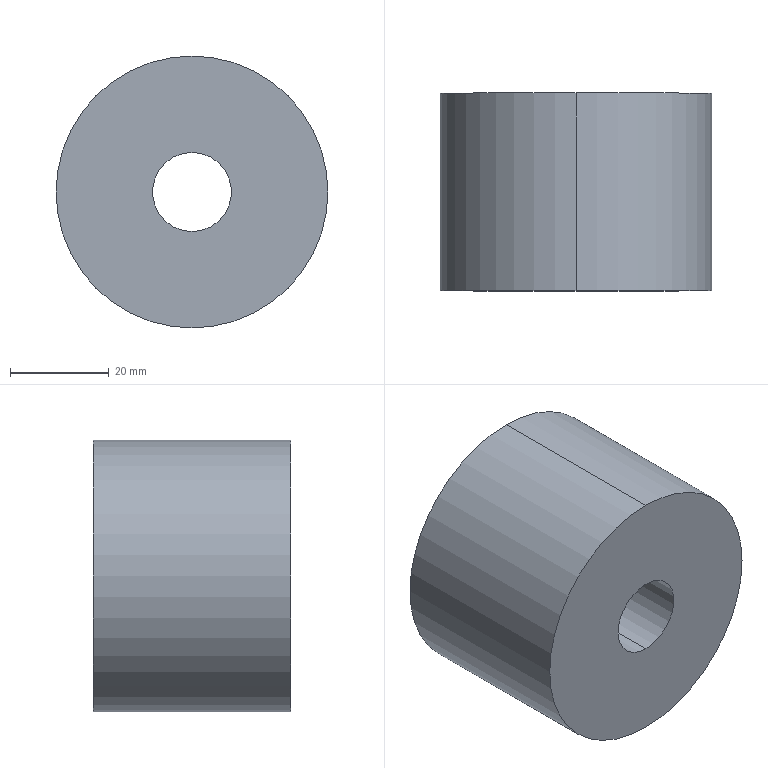Part | STEP file | 19-Limit post | 1 solid | 6 faces | box 55 x 40 x 55 mm | volume 86991 mm3 | cylinder 4 | plane 2 | commonest cylinder face diameters 16 x2 55 x2
STEP:
#1=CARTESIAN_POINT('',(0.,0.,0.));
#2=DIRECTION('',(0.,0.,1.));
#3=DIRECTION('',(1.,0.,0.));
#4=AXIS2_PLACEMENT_3D('',#1,#2,#3);
#5=CARTESIAN_POINT('',(0.,40.,-8.));
#6=VERTEX_POINT('',#5);
#7=CARTESIAN_POINT('',(0.,0.,-8.));
#8=VERTEX_POINT('',#7);
#9=CARTESIAN_POINT('',(0.,40.,-8.));
#10=DIRECTION('',(0.,-1.,0.));
#11=VECTOR('',#10,1.);
#12=LINE('',#9,#11);
#13=CARTESIAN_POINT('',(0.,40.,0.));
#14=DIRECTION('',(0.,-1.,0.));
#15=DIRECTION('',(0.,0.,-1.));
#16=AXIS2_PLACEMENT_3D('',#13,#14,#15);
#17=CYLINDRICAL_SURFACE('',#16,8.);
#18=CARTESIAN_POINT('',(6.283,0.));
#19=DIRECTION('',(0.,1.));
#20=VECTOR('',#19,1.);
#21=LINE('',#18,#20);
#22=(GEOMETRIC_REPRESENTATION_CONTEXT(2)PARAMETRIC_REPRESENTATION_CONTEXT()REPRESENTATION_CONTEXT('',''));
#23=DEFINITIONAL_REPRESENTATION('',(#21),#22);
#24=PCURVE('',#17,#23);
#25=CARTESIAN_POINT('',(0.,40.,0.));
#26=DIRECTION('',(0.,-1.,0.));
#27=DIRECTION('',(0.,0.,-1.));
#28=AXIS2_PLACEMENT_3D('',#25,#26,#27);
#29=CYLINDRICAL_SURFACE('',#28,8.);
#30=CARTESIAN_POINT('',(0.,0.));
#31=DIRECTION('',(0.,1.));
#32=VECTOR('',#31,1.);
#33=LINE('',#30,#32);
#34=(GEOMETRIC_REPRESENTATION_CONTEXT(2)PARAMETRIC_REPRESENTATION_CONTEXT()REPRESENTATION_CONTEXT('',''));
#35=DEFINITIONAL_REPRESENTATION('',(#33),#34);
#36=PCURVE('',#29,#35);
#37=SURFACE_CURVE('',#12,(#24,#36),.PCURVE_S1.);
#38=EDGE_CURVE('',#6,#8,#37,.T.);
#39=ORIENTED_EDGE('',*,*,#38,.T.);
#40=CARTESIAN_POINT('',(0.,0.,8.));
#41=VERTEX_POINT('',#40);
#42=CARTESIAN_POINT('',(0.,0.,0.));
#43=DIRECTION('',(0.,1.,0.));
#44=DIRECTION('',(0.,0.,1.));
#45=AXIS2_PLACEMENT_3D('',#42,#43,#44);
#46=CIRCLE('',#45,8.);
#47=CARTESIAN_POINT('',(9.425,40.));
#48=DIRECTION('',(-1.,0.));
#49=VECTOR('',#48,1.);
#50=LINE('',#47,#49);
#51=(GEOMETRIC_REPRESENTATION_CONTEXT(2)PARAMETRIC_REPRESENTATION_CONTEXT()REPRESENTATION_CONTEXT('',''));
#52=DEFINITIONAL_REPRESENTATION('',(#50),#51);
#53=PCURVE('',#17,#52);
#54=CARTESIAN_POINT('',(0.,0.,0.));
#55=DIRECTION('',(0.,1.,0.));
#56=DIRECTION('',(0.,0.,1.));
#57=AXIS2_PLACEMENT_3D('',#54,#55,#56);
#58=PLANE('',#57);
#59=CARTESIAN_POINT('',(0.,0.));
#60=DIRECTION('',(1.,0.));
#61=AXIS2_PLACEMENT_2D('',#59,#60);
#62=CIRCLE('',#61,8.);
#63=(GEOMETRIC_REPRESENTATION_CONTEXT(2)PARAMETRIC_REPRESENTATION_CONTEXT()REPRESENTATION_CONTEXT('',''));
#64=DEFINITIONAL_REPRESENTATION('',(#62),#63);
#65=PCURVE('',#58,#64);
#66=SURFACE_CURVE('',#46,(#53,#65),.PCURVE_S1.);
#67=EDGE_CURVE('',#8,#41,#66,.T.);
#68=ORIENTED_EDGE('',*,*,#67,.T.);
#69=CARTESIAN_POINT('',(0.,40.,8.));
#70=VERTEX_POINT('',#69);
#71=CARTESIAN_POINT('',(0.,40.,8.));
#72=DIRECTION('',(0.,-1.,0.));
#73=VECTOR('',#72,1.);
#74=LINE('',#71,#73);
#75=CARTESIAN_POINT('',(3.142,0.));
#76=DIRECTION('',(0.,1.));
#77=VECTOR('',#76,1.);
#78=LINE('',#75,#77);
#79=(GEOMETRIC_REPRESENTATION_CONTEXT(2)PARAMETRIC_REPRESENTATION_CONTEXT()REPRESENTATION_CONTEXT('',''));
#80=DEFINITIONAL_REPRESENTATION('',(#78),#79);
#81=PCURVE('',#17,#80);
#82=CARTESIAN_POINT('',(3.142,0.));
#83=DIRECTION('',(0.,1.));
#84=VECTOR('',#83,1.);
#85=LINE('',#82,#84);
#86=(GEOMETRIC_REPRESENTATION_CONTEXT(2)PARAMETRIC_REPRESENTATION_CONTEXT()REPRESENTATION_CONTEXT('',''));
#87=DEFINITIONAL_REPRESENTATION('',(#85),#86);
#88=PCURVE('',#29,#87);
#89=SURFACE_CURVE('',#74,(#81,#88),.PCURVE_S1.);
#90=EDGE_CURVE('',#70,#41,#89,.T.);
#91=ORIENTED_EDGE('',*,*,#90,.F.);
#92=CARTESIAN_POINT('',(0.,40.,0.));
#93=DIRECTION('',(0.,1.,0.));
#94=DIRECTION('',(0.,0.,1.));
#95=AXIS2_PLACEMENT_3D('',#92,#93,#94);
#96=CIRCLE('',#95,8.);
#97=CARTESIAN_POINT('',(9.425,0.));
#98=DIRECTION('',(-1.,0.));
#99=VECTOR('',#98,1.);
#100=LINE('',#97,#99);
#101=(GEOMETRIC_REPRESENTATION_CONTEXT(2)PARAMETRIC_REPRESENTATION_CONTEXT()REPRESENTATION_CONTEXT('',''));
#102=DEFINITIONAL_REPRESENTATION('',(#100),#101);
#103=PCURVE('',#17,#102);
#104=CARTESIAN_POINT('',(0.,40.,0.));
#105=DIRECTION('',(0.,1.,0.));
#106=DIRECTION('',(0.,0.,1.));
#107=AXIS2_PLACEMENT_3D('',#104,#105,#106);
#108=PLANE('',#107);
#109=CARTESIAN_POINT('',(0.,0.));
#110=DIRECTION('',(1.,0.));
#111=AXIS2_PLACEMENT_2D('',#109,#110);
#112=CIRCLE('',#111,8.);
#113=(GEOMETRIC_REPRESENTATION_CONTEXT(2)PARAMETRIC_REPRESENTATION_CONTEXT()REPRESENTATION_CONTEXT('',''));
#114=DEFINITIONAL_REPRESENTATION('',(#112),#113);
#115=PCURVE('',#108,#114);
#116=SURFACE_CURVE('',#96,(#103,#115),.PCURVE_S1.);
#117=EDGE_CURVE('',#6,#70,#116,.T.);
#118=ORIENTED_EDGE('',*,*,#117,.F.);
#119=EDGE_LOOP('',(#39,#68,#91,#118));
#120=FACE_BOUND('',#119,.F.);
#121=ADVANCED_FACE('',(#120),#17,.F.);
#122=CARTESIAN_POINT('',(0.,40.,27.5));
#123=VERTEX_POINT('',#122);
#124=CARTESIAN_POINT('',(0.,40.,-27.5));
#125=VERTEX_POINT('',#124);
#126=CARTESIAN_POINT('',(0.,40.,0.));
#127=DIRECTION('',(0.,1.,0.));
#128=DIRECTION('',(0.,0.,1.));
#129=AXIS2_PLACEMENT_3D('',#126,#127,#128);
#130=CIRCLE('',#129,27.5);
#131=CARTESIAN_POINT('',(0.,40.,0.));
#132=DIRECTION('',(0.,-1.,0.));
#133=DIRECTION('',(0.,0.,-1.));
#134=AXIS2_PLACEMENT_3D('',#131,#132,#133);
#135=CYLINDRICAL_SURFACE('',#134,27.5);
#136=CARTESIAN_POINT('',(3.142,0.));
#137=DIRECTION('',(-1.,0.));
#138=VECTOR('',#137,1.);
#139=LINE('',#136,#138);
#140=(GEOMETRIC_REPRESENTATION_CONTEXT(2)PARAMETRIC_REPRESENTATION_CONTEXT()REPRESENTATION_CONTEXT('',''));
#141=DEFINITIONAL_REPRESENTATION('',(#139),#140);
#142=PCURVE('',#135,#141);
#143=CARTESIAN_POINT('',(0.,0.));
#144=DIRECTION('',(1.,0.));
#145=AXIS2_PLACEMENT_2D('',#143,#144);
#146=CIRCLE('',#145,27.5);
#147=(GEOMETRIC_REPRESENTATION_CONTEXT(2)PARAMETRIC_REPRESENTATION_CONTEXT()REPRESENTATION_CONTEXT('',''));
#148=DEFINITIONAL_REPRESENTATION('',(#146),#147);
#149=PCURVE('',#108,#148);
#150=SURFACE_CURVE('',#130,(#142,#149),.PCURVE_S1.);
#151=EDGE_CURVE('',#123,#125,#150,.T.);
#152=ORIENTED_EDGE('',*,*,#151,.F.);
#153=CARTESIAN_POINT('',(0.,0.,27.5));
#154=VERTEX_POINT('',#153);
#155=CARTESIAN_POINT('',(0.,40.,27.5));
#156=DIRECTION('',(0.,-1.,0.));
#157=VECTOR('',#156,1.);
#158=LINE('',#155,#157);
#159=CARTESIAN_POINT('',(3.142,0.));
#160=DIRECTION('',(0.,1.));
#161=VECTOR('',#160,1.);
#162=LINE('',#159,#161);
#163=(GEOMETRIC_REPRESENTATION_CONTEXT(2)PARAMETRIC_REPRESENTATION_CONTEXT()REPRESENTATION_CONTEXT('',''));
#164=DEFINITIONAL_REPRESENTATION('',(#162),#163);
#165=PCURVE('',#135,#164);
#166=CARTESIAN_POINT('',(0.,40.,0.));
#167=DIRECTION('',(0.,-1.,0.));
#168=DIRECTION('',(0.,0.,-1.));
#169=AXIS2_PLACEMENT_3D('',#166,#167,#168);
#170=CYLINDRICAL_SURFACE('',#169,27.5);
#171=CARTESIAN_POINT('',(3.142,0.));
#172=DIRECTION('',(0.,1.));
#173=VECTOR('',#172,1.);
#174=LINE('',#171,#173);
#175=(GEOMETRIC_REPRESENTATION_CONTEXT(2)PARAMETRIC_REPRESENTATION_CONTEXT()REPRESENTATION_CONTEXT('',''));
#176=DEFINITIONAL_REPRESENTATION('',(#174),#175);
#177=PCURVE('',#170,#176);
#178=SURFACE_CURVE('',#158,(#165,#177),.PCURVE_S1.);
#179=EDGE_CURVE('',#123,#154,#178,.T.);
#180=ORIENTED_EDGE('',*,*,#179,.T.);
#181=CARTESIAN_POINT('',(0.,0.,-27.5));
#182=VERTEX_POINT('',#181);
#183=CARTESIAN_POINT('',(0.,0.,0.));
#184=DIRECTION('',(0.,1.,0.));
#185=DIRECTION('',(0.,0.,1.));
#186=AXIS2_PLACEMENT_3D('',#183,#184,#185);
#187=CIRCLE('',#186,27.5);
#188=CARTESIAN_POINT('',(3.142,40.));
#189=DIRECTION('',(-1.,0.));
#190=VECTOR('',#189,1.);
#191=LINE('',#188,#190);
#192=(GEOMETRIC_REPRESENTATION_CONTEXT(2)PARAMETRIC_REPRESENTATION_CONTEXT()REPRESENTATION_CONTEXT('',''));
#193=DEFINITIONAL_REPRESENTATION('',(#191),#192);
#194=PCURVE('',#135,#193);
#195=CARTESIAN_POINT('',(0.,0.));
#196=DIRECTION('',(1.,0.));
#197=AXIS2_PLACEMENT_2D('',#195,#196);
#198=CIRCLE('',#197,27.5);
#199=(GEOMETRIC_REPRESENTATION_CONTEXT(2)PARAMETRIC_REPRESENTATION_CONTEXT()REPRESENTATION_CONTEXT('',''));
#200=DEFINITIONAL_REPRESENTATION('',(#198),#199);
#201=PCURVE('',#58,#200);
#202=SURFACE_CURVE('',#187,(#194,#201),.PCURVE_S1.);
#203=EDGE_CURVE('',#154,#182,#202,.T.);
#204=ORIENTED_EDGE('',*,*,#203,.T.);
#205=CARTESIAN_POINT('',(0.,40.,-27.5));
#206=DIRECTION('',(0.,-1.,0.));
#207=VECTOR('',#206,1.);
#208=LINE('',#205,#207);
#209=CARTESIAN_POINT('',(0.,0.));
#210=DIRECTION('',(0.,1.));
#211=VECTOR('',#210,1.);
#212=LINE('',#209,#211);
#213=(GEOMETRIC_REPRESENTATION_CONTEXT(2)PARAMETRIC_REPRESENTATION_CONTEXT()REPRESENTATION_CONTEXT('',''));
#214=DEFINITIONAL_REPRESENTATION('',(#212),#213);
#215=PCURVE('',#135,#214);
#216=CARTESIAN_POINT('',(6.283,0.));
#217=DIRECTION('',(0.,1.));
#218=VECTOR('',#217,1.);
#219=LINE('',#216,#218);
#220=(GEOMETRIC_REPRESENTATION_CONTEXT(2)PARAMETRIC_REPRESENTATION_CONTEXT()REPRESENTATION_CONTEXT('',''));
#221=DEFINITIONAL_REPRESENTATION('',(#219),#220);
#222=PCURVE('',#170,#221);
#223=SURFACE_CURVE('',#208,(#215,#222),.PCURVE_S1.);
#224=EDGE_CURVE('',#125,#182,#223,.T.);
#225=ORIENTED_EDGE('',*,*,#224,.F.);
#226=EDGE_LOOP('',(#152,#180,#204,#225));
#227=FACE_BOUND('',#226,.T.);
#228=ADVANCED_FACE('',(#227),#135,.T.);
#229=CARTESIAN_POINT('',(0.,40.,0.));
#230=DIRECTION('',(0.,1.,0.));
#231=DIRECTION('',(0.,0.,1.));
#232=AXIS2_PLACEMENT_3D('',#229,#230,#231);
#233=CIRCLE('',#232,27.5);
#234=CARTESIAN_POINT('',(0.,0.));
#235=DIRECTION('',(1.,0.));
#236=AXIS2_PLACEMENT_2D('',#234,#235);
#237=CIRCLE('',#236,27.5);
#238=(GEOMETRIC_REPRESENTATION_CONTEXT(2)PARAMETRIC_REPRESENTATION_CONTEXT()REPRESENTATION_CONTEXT('',''));
#239=DEFINITIONAL_REPRESENTATION('',(#237),#238);
#240=PCURVE('',#108,#239);
#241=CARTESIAN_POINT('',(9.425,0.));
#242=DIRECTION('',(-1.,0.));
#243=VECTOR('',#242,1.);
#244=LINE('',#241,#243);
#245=(GEOMETRIC_REPRESENTATION_CONTEXT(2)PARAMETRIC_REPRESENTATION_CONTEXT()REPRESENTATION_CONTEXT('',''));
#246=DEFINITIONAL_REPRESENTATION('',(#244),#245);
#247=PCURVE('',#170,#246);
#248=SURFACE_CURVE('',#233,(#240,#247),.PCURVE_S1.);
#249=EDGE_CURVE('',#125,#123,#248,.T.);
#250=ORIENTED_EDGE('',*,*,#249,.T.);
#251=ORIENTED_EDGE('',*,*,#151,.T.);
#252=EDGE_LOOP('',(#250,#251));
#253=FACE_BOUND('',#252,.T.);
#254=ORIENTED_EDGE('',*,*,#117,.F.);
#255=CARTESIAN_POINT('',(0.,40.,0.));
#256=DIRECTION('',(0.,1.,0.));
#257=DIRECTION('',(0.,0.,1.));
#258=AXIS2_PLACEMENT_3D('',#255,#256,#257);
#259=CIRCLE('',#258,8.);
#260=CARTESIAN_POINT('',(0.,0.));
#261=DIRECTION('',(1.,0.));
#262=AXIS2_PLACEMENT_2D('',#260,#261);
#263=CIRCLE('',#262,8.);
#264=(GEOMETRIC_REPRESENTATION_CONTEXT(2)PARAMETRIC_REPRESENTATION_CONTEXT()REPRESENTATION_CONTEXT('',''));
#265=DEFINITIONAL_REPRESENTATION('',(#263),#264);
#266=PCURVE('',#108,#265);
#267=CARTESIAN_POINT('',(3.142,0.));
#268=DIRECTION('',(-1.,0.));
#269=VECTOR('',#268,1.);
#270=LINE('',#267,#269);
#271=(GEOMETRIC_REPRESENTATION_CONTEXT(2)PARAMETRIC_REPRESENTATION_CONTEXT()REPRESENTATION_CONTEXT('',''));
#272=DEFINITIONAL_REPRESENTATION('',(#270),#271);
#273=PCURVE('',#29,#272);
#274=SURFACE_CURVE('',#259,(#266,#273),.PCURVE_S1.);
#275=EDGE_CURVE('',#70,#6,#274,.T.);
#276=ORIENTED_EDGE('',*,*,#275,.F.);
#277=EDGE_LOOP('',(#254,#276));
#278=FACE_BOUND('',#277,.T.);
#279=ADVANCED_FACE('',(#253,#278),#108,.T.);
#280=CARTESIAN_POINT('',(0.,0.,0.));
#281=DIRECTION('',(0.,1.,0.));
#282=DIRECTION('',(0.,0.,1.));
#283=AXIS2_PLACEMENT_3D('',#280,#281,#282);
#284=CIRCLE('',#283,27.5);
#285=CARTESIAN_POINT('',(0.,0.));
#286=DIRECTION('',(1.,0.));
#287=AXIS2_PLACEMENT_2D('',#285,#286);
#288=CIRCLE('',#287,27.5);
#289=(GEOMETRIC_REPRESENTATION_CONTEXT(2)PARAMETRIC_REPRESENTATION_CONTEXT()REPRESENTATION_CONTEXT('',''));
#290=DEFINITIONAL_REPRESENTATION('',(#288),#289);
#291=PCURVE('',#58,#290);
#292=CARTESIAN_POINT('',(9.425,40.));
#293=DIRECTION('',(-1.,0.));
#294=VECTOR('',#293,1.);
#295=LINE('',#292,#294);
#296=(GEOMETRIC_REPRESENTATION_CONTEXT(2)PARAMETRIC_REPRESENTATION_CONTEXT()REPRESENTATION_CONTEXT('',''));
#297=DEFINITIONAL_REPRESENTATION('',(#295),#296);
#298=PCURVE('',#170,#297);
#299=SURFACE_CURVE('',#284,(#291,#298),.PCURVE_S1.);
#300=EDGE_CURVE('',#182,#154,#299,.T.);
#301=ORIENTED_EDGE('',*,*,#300,.F.);
#302=ORIENTED_EDGE('',*,*,#203,.F.);
#303=EDGE_LOOP('',(#301,#302));
#304=FACE_BOUND('',#303,.T.);
#305=ORIENTED_EDGE('',*,*,#67,.T.);
#306=CARTESIAN_POINT('',(0.,0.,0.));
#307=DIRECTION('',(0.,1.,0.));
#308=DIRECTION('',(0.,0.,1.));
#309=AXIS2_PLACEMENT_3D('',#306,#307,#308);
#310=CIRCLE('',#309,8.);
#311=CARTESIAN_POINT('',(0.,0.));
#312=DIRECTION('',(1.,0.));
#313=AXIS2_PLACEMENT_2D('',#311,#312);
#314=CIRCLE('',#313,8.);
#315=(GEOMETRIC_REPRESENTATION_CONTEXT(2)PARAMETRIC_REPRESENTATION_CONTEXT()REPRESENTATION_CONTEXT('',''));
#316=DEFINITIONAL_REPRESENTATION('',(#314),#315);
#317=PCURVE('',#58,#316);
#318=CARTESIAN_POINT('',(3.142,40.));
#319=DIRECTION('',(-1.,0.));
#320=VECTOR('',#319,1.);
#321=LINE('',#318,#320);
#322=(GEOMETRIC_REPRESENTATION_CONTEXT(2)PARAMETRIC_REPRESENTATION_CONTEXT()REPRESENTATION_CONTEXT('',''));
#323=DEFINITIONAL_REPRESENTATION('',(#321),#322);
#324=PCURVE('',#29,#323);
#325=SURFACE_CURVE('',#310,(#317,#324),.PCURVE_S1.);
#326=EDGE_CURVE('',#41,#8,#325,.T.);
#327=ORIENTED_EDGE('',*,*,#326,.T.);
#328=EDGE_LOOP('',(#305,#327));
#329=FACE_BOUND('',#328,.T.);
#330=ADVANCED_FACE('',(#304,#329),#58,.F.);
#331=ORIENTED_EDGE('',*,*,#179,.F.);
#332=ORIENTED_EDGE('',*,*,#249,.F.);
#333=ORIENTED_EDGE('',*,*,#224,.T.);
#334=ORIENTED_EDGE('',*,*,#300,.T.);
#335=EDGE_LOOP('',(#331,#332,#333,#334));
#336=FACE_BOUND('',#335,.T.);
#337=ADVANCED_FACE('',(#336),#170,.T.);
#338=ORIENTED_EDGE('',*,*,#326,.T.);
#339=ORIENTED_EDGE('',*,*,#38,.F.);
#340=ORIENTED_EDGE('',*,*,#275,.F.);
#341=ORIENTED_EDGE('',*,*,#90,.T.);
#342=EDGE_LOOP('',(#338,#339,#340,#341));
#343=FACE_BOUND('',#342,.F.);
#344=ADVANCED_FACE('',(#343),#29,.F.);
#345=CLOSED_SHELL('',(#121,#228,#279,#330,#337,#344));
#346=MANIFOLD_SOLID_BREP('',#345);
#347=(LENGTH_UNIT()NAMED_UNIT(*)SI_UNIT(.MILLI.,.METRE.));
#348=UNCERTAINTY_MEASURE_WITH_UNIT(LENGTH_MEASURE(0.0000001),#347,'','');
#349=(NAMED_UNIT(*)PLANE_ANGLE_UNIT()SI_UNIT($,.RADIAN.));
#350=(NAMED_UNIT(*)SI_UNIT($,.STERADIAN.)SOLID_ANGLE_UNIT());
#351=(GEOMETRIC_REPRESENTATION_CONTEXT(3)GLOBAL_UNCERTAINTY_ASSIGNED_CONTEXT((#348))GLOBAL_UNIT_ASSIGNED_CONTEXT((#347,#349,#350))REPRESENTATION_CONTEXT('',''));
#352=ADVANCED_BREP_SHAPE_REPRESENTATION('',(#4,#346),#351);